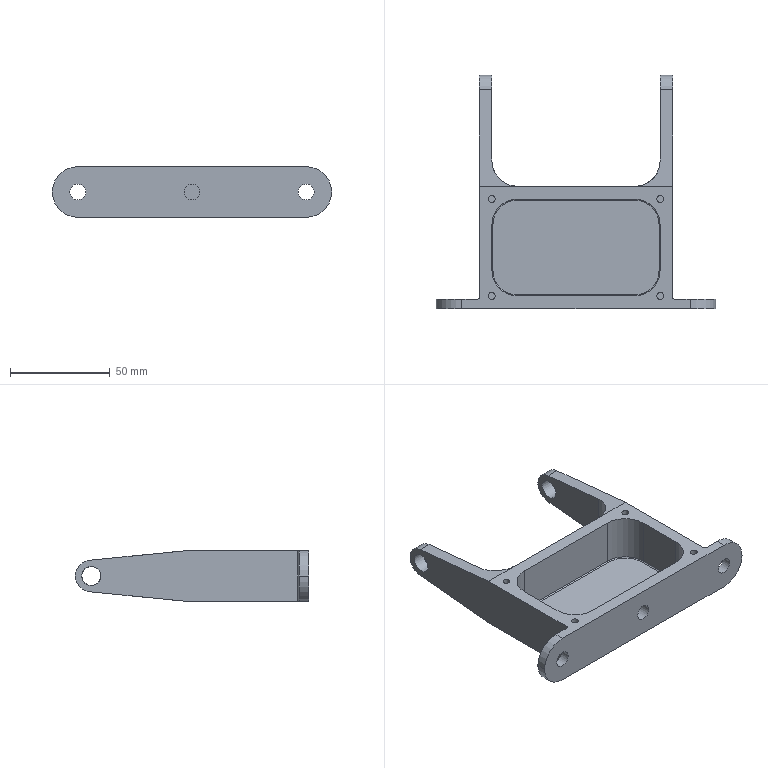Part | NX | features MG0330 trunion parts 24(steering fork) 2 | 1 solid | 54 faces | box 139.7 x 116.681 x 25.4 mm | volume 74432 mm3 | cylinder 27 | plane 23 | torus 4 | commonest cylinder face diameters 25.4 x10 1.016 x4 3.454 x4 7.938 x3 1.524 x2 9.525 x2
STEP:
#1=CARTESIAN_POINT('',(-29.369,-60.325,12.7));
#2=VERTEX_POINT('',#1);
#3=CARTESIAN_POINT('',(-29.369,-60.325,-10.617));
#4=VERTEX_POINT('',#3);
#5=CARTESIAN_POINT('',(-29.369,-60.325,-11.125));
#6=DIRECTION('',(0.,0.,-1.));
#7=VECTOR('',#6,1000.);
#8=LINE('',#5,#7);
#9=EDGE_CURVE('',#2,#4,#8,.T.);
#10=ORIENTED_EDGE('',*,*,#9,.T.);
#11=CARTESIAN_POINT('',(29.369,-60.325,-10.617));
#12=VERTEX_POINT('',#11);
#13=CARTESIAN_POINT('',(29.369,-60.325,-10.617));
#14=DIRECTION('',(1.,0.,0.));
#15=VECTOR('',#14,1000.);
#16=LINE('',#13,#15);
#17=EDGE_CURVE('',#4,#12,#16,.T.);
#18=ORIENTED_EDGE('',*,*,#17,.T.);
#19=CARTESIAN_POINT('',(29.369,-60.325,12.7));
#20=VERTEX_POINT('',#19);
#21=CARTESIAN_POINT('',(29.369,-60.325,12.7));
#22=DIRECTION('',(0.,0.,-1.));
#23=VECTOR('',#22,1000.);
#24=LINE('',#21,#23);
#25=EDGE_CURVE('',#12,#20,#24,.F.);
#26=ORIENTED_EDGE('',*,*,#25,.T.);
#27=CARTESIAN_POINT('',(42.069,-60.325,12.7));
#28=DIRECTION('',(1.,0.,0.));
#29=VECTOR('',#28,1000.);
#30=LINE('',#27,#29);
#31=EDGE_CURVE('',#2,#20,#30,.T.);
#32=ORIENTED_EDGE('',*,*,#31,.F.);
#33=EDGE_LOOP('',(#10,#18,#26,#32));
#34=FACE_BOUND('',#33,.T.);
#35=CARTESIAN_POINT('',(42.069,-60.325,12.7));
#36=DIRECTION('',(0.,1.,0.));
#37=DIRECTION('',(0.,0.,1.));
#38=AXIS2_PLACEMENT_3D('',#35,#36,#37);
#39=PLANE('',#38);
#40=ADVANCED_FACE('',(#34),#39,.F.);
#41=CARTESIAN_POINT('',(42.069,-73.025,12.7));
#42=VERTEX_POINT('',#41);
#43=CARTESIAN_POINT('',(42.069,-73.025,-10.617));
#44=VERTEX_POINT('',#43);
#45=CARTESIAN_POINT('',(42.069,-73.025,-11.125));
#46=DIRECTION('',(0.,0.,-1.));
#47=VECTOR('',#46,1000.);
#48=LINE('',#45,#47);
#49=EDGE_CURVE('',#42,#44,#48,.T.);
#50=ORIENTED_EDGE('',*,*,#49,.T.);
#51=CARTESIAN_POINT('',(42.069,-96.044,-10.617));
#52=VERTEX_POINT('',#51);
#53=CARTESIAN_POINT('',(42.069,-96.044,-10.617));
#54=DIRECTION('',(0.,-1.,0.));
#55=VECTOR('',#54,1000.);
#56=LINE('',#53,#55);
#57=EDGE_CURVE('',#44,#52,#56,.T.);
#58=ORIENTED_EDGE('',*,*,#57,.T.);
#59=CARTESIAN_POINT('',(42.069,-96.044,12.7));
#60=VERTEX_POINT('',#59);
#61=CARTESIAN_POINT('',(42.069,-96.044,12.7));
#62=DIRECTION('',(0.,0.,-1.));
#63=VECTOR('',#62,1000.);
#64=LINE('',#61,#63);
#65=EDGE_CURVE('',#52,#60,#64,.F.);
#66=ORIENTED_EDGE('',*,*,#65,.T.);
#67=CARTESIAN_POINT('',(42.069,-60.325,12.7));
#68=DIRECTION('',(0.,-1.,0.));
#69=VECTOR('',#68,1000.);
#70=LINE('',#67,#69);
#71=EDGE_CURVE('',#42,#60,#70,.T.);
#72=ORIENTED_EDGE('',*,*,#71,.F.);
#73=EDGE_LOOP('',(#50,#58,#66,#72));
#74=FACE_BOUND('',#73,.T.);
#75=CARTESIAN_POINT('',(42.069,-60.325,12.7));
#76=DIRECTION('',(1.,0.,0.));
#77=DIRECTION('',(0.,1.,0.));
#78=AXIS2_PLACEMENT_3D('',#75,#76,#77);
#79=PLANE('',#78);
#80=ADVANCED_FACE('',(#74),#79,.F.);
#81=CARTESIAN_POINT('',(0.,-108.744,-3.969));
#82=VERTEX_POINT('',#81);
#83=CARTESIAN_POINT('',(0.,-108.744,0.));
#84=DIRECTION('',(0.,-1.,0.));
#85=DIRECTION('',(0.,0.,-1.));
#86=AXIS2_PLACEMENT_3D('',#83,#84,#85);
#87=CIRCLE('',#86,3.969);
#88=EDGE_CURVE('',#82,#82,#87,.F.);
#89=ORIENTED_EDGE('',*,*,#88,.F.);
#90=EDGE_LOOP('',(#89));
#91=FACE_BOUND('',#90,.T.);
#92=CARTESIAN_POINT('',(29.369,-108.744,12.7));
#93=VERTEX_POINT('',#92);
#94=CARTESIAN_POINT('',(29.369,-108.744,-10.617));
#95=VERTEX_POINT('',#94);
#96=CARTESIAN_POINT('',(29.369,-108.744,-11.125));
#97=DIRECTION('',(0.,0.,-1.));
#98=VECTOR('',#97,1000.);
#99=LINE('',#96,#98);
#100=EDGE_CURVE('',#93,#95,#99,.T.);
#101=ORIENTED_EDGE('',*,*,#100,.T.);
#102=CARTESIAN_POINT('',(-29.369,-108.744,-10.617));
#103=VERTEX_POINT('',#102);
#104=CARTESIAN_POINT('',(-29.369,-108.744,-10.617));
#105=DIRECTION('',(-1.,0.,0.));
#106=VECTOR('',#105,1000.);
#107=LINE('',#104,#106);
#108=EDGE_CURVE('',#95,#103,#107,.T.);
#109=ORIENTED_EDGE('',*,*,#108,.T.);
#110=CARTESIAN_POINT('',(-29.369,-108.744,12.7));
#111=VERTEX_POINT('',#110);
#112=CARTESIAN_POINT('',(-29.369,-108.744,12.7));
#113=DIRECTION('',(0.,0.,-1.));
#114=VECTOR('',#113,1000.);
#115=LINE('',#112,#114);
#116=EDGE_CURVE('',#103,#111,#115,.F.);
#117=ORIENTED_EDGE('',*,*,#116,.T.);
#118=CARTESIAN_POINT('',(42.069,-108.744,12.7));
#119=DIRECTION('',(-1.,0.,0.));
#120=VECTOR('',#119,1000.);
#121=LINE('',#118,#120);
#122=EDGE_CURVE('',#93,#111,#121,.T.);
#123=ORIENTED_EDGE('',*,*,#122,.F.);
#124=EDGE_LOOP('',(#101,#109,#117,#123));
#125=FACE_BOUND('',#124,.T.);
#126=CARTESIAN_POINT('',(42.069,-108.744,12.7));
#127=DIRECTION('',(0.,-1.,0.));
#128=DIRECTION('',(0.,0.,-1.));
#129=AXIS2_PLACEMENT_3D('',#126,#127,#128);
#130=PLANE('',#129);
#131=ADVANCED_FACE('',(#91,#125),#130,.F.);
#132=CARTESIAN_POINT('',(57.15,-115.094,-3.969));
#133=VERTEX_POINT('',#132);
#134=CARTESIAN_POINT('',(57.15,-115.094,0.));
#135=DIRECTION('',(0.,-1.,0.));
#136=DIRECTION('',(0.,0.,-1.));
#137=AXIS2_PLACEMENT_3D('',#134,#135,#136);
#138=CIRCLE('',#137,3.969);
#139=EDGE_CURVE('',#133,#133,#138,.T.);
#140=ORIENTED_EDGE('',*,*,#139,.F.);
#141=EDGE_LOOP('',(#140));
#142=FACE_BOUND('',#141,.T.);
#143=CARTESIAN_POINT('',(-57.15,-115.094,-3.969));
#144=VERTEX_POINT('',#143);
#145=CARTESIAN_POINT('',(-57.15,-115.094,0.));
#146=DIRECTION('',(0.,-1.,0.));
#147=DIRECTION('',(0.,0.,-1.));
#148=AXIS2_PLACEMENT_3D('',#145,#146,#147);
#149=CIRCLE('',#148,3.969);
#150=EDGE_CURVE('',#144,#144,#149,.T.);
#151=ORIENTED_EDGE('',*,*,#150,.F.);
#152=EDGE_LOOP('',(#151));
#153=FACE_BOUND('',#152,.T.);
#154=CARTESIAN_POINT('',(0.,-115.094,-3.969));
#155=VERTEX_POINT('',#154);
#156=CARTESIAN_POINT('',(0.,-115.094,0.));
#157=DIRECTION('',(0.,-1.,0.));
#158=DIRECTION('',(0.,0.,-1.));
#159=AXIS2_PLACEMENT_3D('',#156,#157,#158);
#160=CIRCLE('',#159,3.969);
#161=EDGE_CURVE('',#155,#155,#160,.T.);
#162=ORIENTED_EDGE('',*,*,#161,.F.);
#163=EDGE_LOOP('',(#162));
#164=FACE_BOUND('',#163,.T.);
#165=CARTESIAN_POINT('',(-57.15,-115.094,12.7));
#166=VERTEX_POINT('',#165);
#167=CARTESIAN_POINT('',(-69.85,-115.094,0.));
#168=VERTEX_POINT('',#167);
#169=CARTESIAN_POINT('',(-57.15,-115.094,0.));
#170=DIRECTION('',(0.,1.,0.));
#171=DIRECTION('',(-1.,0.,0.));
#172=AXIS2_PLACEMENT_3D('',#169,#170,#171);
#173=CIRCLE('',#172,12.7);
#174=EDGE_CURVE('',#166,#168,#173,.F.);
#175=ORIENTED_EDGE('',*,*,#174,.T.);
#176=CARTESIAN_POINT('',(-57.15,-115.094,-12.7));
#177=VERTEX_POINT('',#176);
#178=CARTESIAN_POINT('',(-57.15,-115.094,0.));
#179=DIRECTION('',(0.,1.,0.));
#180=DIRECTION('',(-1.,0.,0.));
#181=AXIS2_PLACEMENT_3D('',#178,#179,#180);
#182=CIRCLE('',#181,12.7);
#183=EDGE_CURVE('',#168,#177,#182,.F.);
#184=ORIENTED_EDGE('',*,*,#183,.T.);
#185=CARTESIAN_POINT('',(57.15,-115.094,-12.7));
#186=VERTEX_POINT('',#185);
#187=CARTESIAN_POINT('',(0.,-115.094,-12.7));
#188=DIRECTION('',(1.,0.,0.));
#189=VECTOR('',#188,1000.);
#190=LINE('',#187,#189);
#191=EDGE_CURVE('',#177,#186,#190,.T.);
#192=ORIENTED_EDGE('',*,*,#191,.T.);
#193=CARTESIAN_POINT('',(69.85,-115.094,0.));
#194=VERTEX_POINT('',#193);
#195=CARTESIAN_POINT('',(57.15,-115.094,0.));
#196=DIRECTION('',(0.,1.,0.));
#197=DIRECTION('',(-1.,0.,0.));
#198=AXIS2_PLACEMENT_3D('',#195,#196,#197);
#199=CIRCLE('',#198,12.7);
#200=EDGE_CURVE('',#186,#194,#199,.F.);
#201=ORIENTED_EDGE('',*,*,#200,.T.);
#202=CARTESIAN_POINT('',(57.15,-115.094,12.7));
#203=VERTEX_POINT('',#202);
#204=CARTESIAN_POINT('',(57.15,-115.094,0.));
#205=DIRECTION('',(0.,1.,0.));
#206=DIRECTION('',(-1.,0.,0.));
#207=AXIS2_PLACEMENT_3D('',#204,#205,#206);
#208=CIRCLE('',#207,12.7);
#209=EDGE_CURVE('',#194,#203,#208,.F.);
#210=ORIENTED_EDGE('',*,*,#209,.T.);
#211=CARTESIAN_POINT('',(0.,-115.094,12.7));
#212=DIRECTION('',(1.,0.,0.));
#213=VECTOR('',#212,1000.);
#214=LINE('',#211,#213);
#215=EDGE_CURVE('',#166,#203,#214,.T.);
#216=ORIENTED_EDGE('',*,*,#215,.F.);
#217=EDGE_LOOP('',(#175,#184,#192,#201,#210,#216));
#218=FACE_BOUND('',#217,.T.);
#219=CARTESIAN_POINT('',(0.,-115.094,12.7));
#220=DIRECTION('',(0.,1.,0.));
#221=DIRECTION('',(-1.,0.,0.));
#222=AXIS2_PLACEMENT_3D('',#219,#220,#221);
#223=PLANE('',#222);
#224=ADVANCED_FACE('',(#142,#153,#164,#218),#223,.F.);
#225=CARTESIAN_POINT('',(57.15,-110.331,-3.969));
#226=VERTEX_POINT('',#225);
#227=CARTESIAN_POINT('',(57.15,-110.331,0.));
#228=DIRECTION('',(0.,-1.,0.));
#229=DIRECTION('',(0.,0.,-1.));
#230=AXIS2_PLACEMENT_3D('',#227,#228,#229);
#231=CIRCLE('',#230,3.969);
#232=EDGE_CURVE('',#226,#226,#231,.T.);
#233=ORIENTED_EDGE('',*,*,#232,.T.);
#234=EDGE_LOOP('',(#233));
#235=FACE_BOUND('',#234,.T.);
#236=CARTESIAN_POINT('',(57.15,-110.331,-12.7));
#237=VERTEX_POINT('',#236);
#238=CARTESIAN_POINT('',(49.181,-110.331,-12.7));
#239=VERTEX_POINT('',#238);
#240=CARTESIAN_POINT('',(69.85,-110.331,-12.7));
#241=DIRECTION('',(-1.,0.,0.));
#242=VECTOR('',#241,1000.);
#243=LINE('',#240,#242);
#244=EDGE_CURVE('',#237,#239,#243,.T.);
#245=ORIENTED_EDGE('',*,*,#244,.T.);
#246=CARTESIAN_POINT('',(49.181,-110.331,12.7));
#247=VERTEX_POINT('',#246);
#248=CARTESIAN_POINT('',(49.181,-110.331,12.7));
#249=DIRECTION('',(0.,0.,-1.));
#250=VECTOR('',#249,1000.);
#251=LINE('',#248,#250);
#252=EDGE_CURVE('',#239,#247,#251,.F.);
#253=ORIENTED_EDGE('',*,*,#252,.T.);
#254=CARTESIAN_POINT('',(57.15,-110.331,12.7));
#255=VERTEX_POINT('',#254);
#256=CARTESIAN_POINT('',(69.85,-110.331,12.7));
#257=DIRECTION('',(-1.,0.,0.));
#258=VECTOR('',#257,1000.);
#259=LINE('',#256,#258);
#260=EDGE_CURVE('',#255,#247,#259,.T.);
#261=ORIENTED_EDGE('',*,*,#260,.F.);
#262=CARTESIAN_POINT('',(69.85,-110.331,0.));
#263=VERTEX_POINT('',#262);
#264=CARTESIAN_POINT('',(57.15,-110.331,0.));
#265=DIRECTION('',(0.,-1.,0.));
#266=DIRECTION('',(0.,0.,-1.));
#267=AXIS2_PLACEMENT_3D('',#264,#265,#266);
#268=CIRCLE('',#267,12.7);
#269=EDGE_CURVE('',#255,#263,#268,.F.);
#270=ORIENTED_EDGE('',*,*,#269,.T.);
#271=CARTESIAN_POINT('',(57.15,-110.331,0.));
#272=DIRECTION('',(0.,-1.,0.));
#273=DIRECTION('',(0.,0.,-1.));
#274=AXIS2_PLACEMENT_3D('',#271,#272,#273);
#275=CIRCLE('',#274,12.7);
#276=EDGE_CURVE('',#263,#237,#275,.F.);
#277=ORIENTED_EDGE('',*,*,#276,.T.);
#278=EDGE_LOOP('',(#245,#253,#261,#270,#277));
#279=FACE_BOUND('',#278,.T.);
#280=CARTESIAN_POINT('',(69.85,-110.331,12.7));
#281=DIRECTION('',(0.,-1.,0.));
#282=DIRECTION('',(0.,0.,-1.));
#283=AXIS2_PLACEMENT_3D('',#280,#281,#282);
#284=PLANE('',#283);
#285=ADVANCED_FACE('',(#235,#279),#284,.F.);
#286=CARTESIAN_POINT('',(48.419,-6.35,4.763));
#287=VERTEX_POINT('',#286);
#288=CARTESIAN_POINT('',(48.419,-6.35,0.));
#289=DIRECTION('',(-1.,0.,0.));
#290=DIRECTION('',(0.,0.,1.));
#291=AXIS2_PLACEMENT_3D('',#288,#289,#290);
#292=CIRCLE('',#291,4.763);
#293=EDGE_CURVE('',#287,#287,#292,.T.);
#294=ORIENTED_EDGE('',*,*,#293,.T.);
#295=EDGE_LOOP('',(#294));
#296=FACE_BOUND('',#295,.T.);
#297=CARTESIAN_POINT('',(48.419,-109.569,12.7));
#298=VERTEX_POINT('',#297);
#299=CARTESIAN_POINT('',(48.419,-53.975,12.7));
#300=VERTEX_POINT('',#299);
#301=CARTESIAN_POINT('',(48.419,-110.331,12.7));
#302=DIRECTION('',(0.,1.,0.));
#303=VECTOR('',#302,1000.);
#304=LINE('',#301,#303);
#305=EDGE_CURVE('',#298,#300,#304,.T.);
#306=ORIENTED_EDGE('',*,*,#305,.F.);
#307=CARTESIAN_POINT('',(48.419,-109.569,-12.7));
#308=VERTEX_POINT('',#307);
#309=CARTESIAN_POINT('',(48.419,-109.569,-12.7));
#310=DIRECTION('',(0.,0.,-1.));
#311=VECTOR('',#310,1000.);
#312=LINE('',#309,#311);
#313=EDGE_CURVE('',#298,#308,#312,.T.);
#314=ORIENTED_EDGE('',*,*,#313,.T.);
#315=CARTESIAN_POINT('',(48.419,-53.975,-12.7));
#316=VERTEX_POINT('',#315);
#317=CARTESIAN_POINT('',(48.419,-110.331,-12.7));
#318=DIRECTION('',(0.,1.,0.));
#319=VECTOR('',#318,1000.);
#320=LINE('',#317,#319);
#321=EDGE_CURVE('',#308,#316,#320,.T.);
#322=ORIENTED_EDGE('',*,*,#321,.T.);
#323=CARTESIAN_POINT('',(48.419,-5.567,-7.899));
#324=VERTEX_POINT('',#323);
#325=CARTESIAN_POINT('',(48.419,-107.288,-17.988));
#326=DIRECTION('',(0.,0.9951,0.0987));
#327=VECTOR('',#326,1000.);
#328=LINE('',#325,#327);
#329=EDGE_CURVE('',#316,#324,#328,.T.);
#330=ORIENTED_EDGE('',*,*,#329,.T.);
#331=CARTESIAN_POINT('',(48.419,-5.567,7.899));
#332=VERTEX_POINT('',#331);
#333=CARTESIAN_POINT('',(48.419,-6.35,0.));
#334=DIRECTION('',(-1.,0.,0.));
#335=DIRECTION('',(0.,0.,1.));
#336=AXIS2_PLACEMENT_3D('',#333,#334,#335);
#337=CIRCLE('',#336,7.938);
#338=EDGE_CURVE('',#324,#332,#337,.F.);
#339=ORIENTED_EDGE('',*,*,#338,.T.);
#340=CARTESIAN_POINT('',(48.419,-109.782,18.235));
#341=DIRECTION('',(0.,-0.9951,0.0987));
#342=VECTOR('',#341,1000.);
#343=LINE('',#340,#342);
#344=EDGE_CURVE('',#332,#300,#343,.T.);
#345=ORIENTED_EDGE('',*,*,#344,.T.);
#346=EDGE_LOOP('',(#306,#314,#322,#330,#339,#345));
#347=FACE_BOUND('',#346,.T.);
#348=CARTESIAN_POINT('',(48.419,-110.331,12.7));
#349=DIRECTION('',(-1.,0.,0.));
#350=DIRECTION('',(0.,0.,1.));
#351=AXIS2_PLACEMENT_3D('',#348,#349,#350);
#352=PLANE('',#351);
#353=ADVANCED_FACE('',(#296,#347),#352,.F.);
#354=CARTESIAN_POINT('',(42.069,-1.587,0.));
#355=VERTEX_POINT('',#354);
#356=CARTESIAN_POINT('',(42.069,-6.35,0.));
#357=DIRECTION('',(1.,0.,0.));
#358=DIRECTION('',(0.,1.,0.));
#359=AXIS2_PLACEMENT_3D('',#356,#357,#358);
#360=CIRCLE('',#359,4.763);
#361=EDGE_CURVE('',#355,#355,#360,.T.);
#362=ORIENTED_EDGE('',*,*,#361,.T.);
#363=EDGE_LOOP('',(#362));
#364=FACE_BOUND('',#363,.T.);
#365=CARTESIAN_POINT('',(42.069,-5.567,7.899));
#366=VERTEX_POINT('',#365);
#367=CARTESIAN_POINT('',(42.069,-5.567,-7.899));
#368=VERTEX_POINT('',#367);
#369=CARTESIAN_POINT('',(42.069,-6.35,0.));
#370=DIRECTION('',(1.,0.,0.));
#371=DIRECTION('',(0.,1.,0.));
#372=AXIS2_PLACEMENT_3D('',#369,#370,#371);
#373=CIRCLE('',#372,7.938);
#374=EDGE_CURVE('',#366,#368,#373,.F.);
#375=ORIENTED_EDGE('',*,*,#374,.T.);
#376=CARTESIAN_POINT('',(42.069,-41.275,-11.44));
#377=VERTEX_POINT('',#376);
#378=CARTESIAN_POINT('',(42.069,5.113,-6.84));
#379=DIRECTION('',(0.,-0.9951,-0.0987));
#380=VECTOR('',#379,1000.);
#381=LINE('',#378,#380);
#382=EDGE_CURVE('',#368,#377,#381,.T.);
#383=ORIENTED_EDGE('',*,*,#382,.T.);
#384=CARTESIAN_POINT('',(42.069,-41.275,11.44));
#385=VERTEX_POINT('',#384);
#386=CARTESIAN_POINT('',(42.069,-41.275,12.7));
#387=DIRECTION('',(0.,0.,-1.));
#388=VECTOR('',#387,1000.);
#389=LINE('',#386,#388);
#390=EDGE_CURVE('',#377,#385,#389,.F.);
#391=ORIENTED_EDGE('',*,*,#390,.T.);
#392=CARTESIAN_POINT('',(42.069,2.618,7.087));
#393=DIRECTION('',(0.,0.9951,-0.0987));
#394=VECTOR('',#393,1000.);
#395=LINE('',#392,#394);
#396=EDGE_CURVE('',#385,#366,#395,.T.);
#397=ORIENTED_EDGE('',*,*,#396,.T.);
#398=EDGE_LOOP('',(#375,#383,#391,#397));
#399=FACE_BOUND('',#398,.T.);
#400=CARTESIAN_POINT('',(42.069,3.175,12.7));
#401=DIRECTION('',(1.,0.,0.));
#402=DIRECTION('',(0.,1.,0.));
#403=AXIS2_PLACEMENT_3D('',#400,#401,#402);
#404=PLANE('',#403);
#405=ADVANCED_FACE('',(#364,#399),#404,.F.);
#406=CARTESIAN_POINT('',(29.369,-53.975,12.7));
#407=VERTEX_POINT('',#406);
#408=CARTESIAN_POINT('',(-29.369,-53.975,12.7));
#409=VERTEX_POINT('',#408);
#410=CARTESIAN_POINT('',(42.069,-53.975,12.7));
#411=DIRECTION('',(-1.,0.,0.));
#412=VECTOR('',#411,1000.);
#413=LINE('',#410,#412);
#414=EDGE_CURVE('',#407,#409,#413,.T.);
#415=ORIENTED_EDGE('',*,*,#414,.F.);
#416=CARTESIAN_POINT('',(29.369,-53.975,-12.7));
#417=VERTEX_POINT('',#416);
#418=CARTESIAN_POINT('',(29.369,-53.975,-12.7));
#419=DIRECTION('',(0.,0.,-1.));
#420=VECTOR('',#419,1000.);
#421=LINE('',#418,#420);
#422=EDGE_CURVE('',#407,#417,#421,.T.);
#423=ORIENTED_EDGE('',*,*,#422,.T.);
#424=CARTESIAN_POINT('',(-29.369,-53.975,-12.7));
#425=VERTEX_POINT('',#424);
#426=CARTESIAN_POINT('',(42.069,-53.975,-12.7));
#427=DIRECTION('',(-1.,0.,0.));
#428=VECTOR('',#427,1000.);
#429=LINE('',#426,#428);
#430=EDGE_CURVE('',#417,#425,#429,.T.);
#431=ORIENTED_EDGE('',*,*,#430,.T.);
#432=CARTESIAN_POINT('',(-29.369,-53.975,12.7));
#433=DIRECTION('',(0.,0.,-1.));
#434=VECTOR('',#433,1000.);
#435=LINE('',#432,#434);
#436=EDGE_CURVE('',#425,#409,#435,.F.);
#437=ORIENTED_EDGE('',*,*,#436,.T.);
#438=EDGE_LOOP('',(#415,#423,#431,#437));
#439=FACE_BOUND('',#438,.T.);
#440=CARTESIAN_POINT('',(42.069,-53.975,12.7));
#441=DIRECTION('',(0.,-1.,0.));
#442=DIRECTION('',(1.,0.,0.));
#443=AXIS2_PLACEMENT_3D('',#440,#441,#442);
#444=PLANE('',#443);
#445=ADVANCED_FACE('',(#439),#444,.F.);
#446=CARTESIAN_POINT('',(-43.796,-60.325,12.7));
#447=VERTEX_POINT('',#446);
#448=CARTESIAN_POINT('',(-42.069,-60.325,12.7));
#449=DIRECTION('',(0.,0.,-1.));
#450=DIRECTION('',(-1.,0.,0.));
#451=AXIS2_PLACEMENT_3D('',#448,#449,#450);
#452=CIRCLE('',#451,1.727);
#453=EDGE_CURVE('',#447,#447,#452,.F.);
#454=ORIENTED_EDGE('',*,*,#453,.F.);
#455=EDGE_LOOP('',(#454));
#456=FACE_BOUND('',#455,.T.);
#457=CARTESIAN_POINT('',(40.342,-60.325,12.7));
#458=VERTEX_POINT('',#457);
#459=CARTESIAN_POINT('',(42.069,-60.325,12.7));
#460=DIRECTION('',(0.,0.,-1.));
#461=DIRECTION('',(-1.,0.,0.));
#462=AXIS2_PLACEMENT_3D('',#459,#460,#461);
#463=CIRCLE('',#462,1.727);
#464=EDGE_CURVE('',#458,#458,#463,.F.);
#465=ORIENTED_EDGE('',*,*,#464,.F.);
#466=EDGE_LOOP('',(#465));
#467=FACE_BOUND('',#466,.T.);
#468=CARTESIAN_POINT('',(40.342,-108.744,12.7));
#469=VERTEX_POINT('',#468);
#470=CARTESIAN_POINT('',(42.069,-108.744,12.7));
#471=DIRECTION('',(0.,0.,-1.));
#472=DIRECTION('',(-1.,0.,0.));
#473=AXIS2_PLACEMENT_3D('',#470,#471,#472);
#474=CIRCLE('',#473,1.727);
#475=EDGE_CURVE('',#469,#469,#474,.F.);
#476=ORIENTED_EDGE('',*,*,#475,.F.);
#477=EDGE_LOOP('',(#476));
#478=FACE_BOUND('',#477,.T.);
#479=CARTESIAN_POINT('',(-43.796,-108.744,12.7));
#480=VERTEX_POINT('',#479);
#481=CARTESIAN_POINT('',(-42.069,-108.744,12.7));
#482=DIRECTION('',(0.,0.,-1.));
#483=DIRECTION('',(-1.,0.,0.));
#484=AXIS2_PLACEMENT_3D('',#481,#482,#483);
#485=CIRCLE('',#484,1.727);
#486=EDGE_CURVE('',#480,#480,#485,.F.);
#487=ORIENTED_EDGE('',*,*,#486,.F.);
#488=EDGE_LOOP('',(#487));
#489=FACE_BOUND('',#488,.T.);
#490=ORIENTED_EDGE('',*,*,#260,.T.);
#491=CARTESIAN_POINT('',(49.181,-109.569,12.7));
#492=DIRECTION('',(0.,0.,-1.));
#493=DIRECTION('',(-1.,0.,0.));
#494=AXIS2_PLACEMENT_3D('',#491,#492,#493);
#495=CIRCLE('',#494,0.762);
#496=EDGE_CURVE('',#247,#298,#495,.T.);
#497=ORIENTED_EDGE('',*,*,#496,.T.);
#498=ORIENTED_EDGE('',*,*,#305,.T.);
#499=CARTESIAN_POINT('',(590.751,-53.975,12.7));
#500=DIRECTION('',(-1.,0.,0.));
#501=VECTOR('',#500,1000.);
#502=LINE('',#499,#501);
#503=EDGE_CURVE('',#300,#407,#502,.T.);
#504=ORIENTED_EDGE('',*,*,#503,.T.);
#505=ORIENTED_EDGE('',*,*,#414,.T.);
#506=CARTESIAN_POINT('',(-48.419,-53.975,12.7));
#507=VERTEX_POINT('',#506);
#508=CARTESIAN_POINT('',(590.751,-53.975,12.7));
#509=DIRECTION('',(-1.,0.,0.));
#510=VECTOR('',#509,1000.);
#511=LINE('',#508,#510);
#512=EDGE_CURVE('',#409,#507,#511,.T.);
#513=ORIENTED_EDGE('',*,*,#512,.T.);
#514=CARTESIAN_POINT('',(-48.419,-109.569,12.7));
#515=VERTEX_POINT('',#514);
#516=CARTESIAN_POINT('',(-48.419,-110.331,12.7));
#517=DIRECTION('',(0.,1.,0.));
#518=VECTOR('',#517,1000.);
#519=LINE('',#516,#518);
#520=EDGE_CURVE('',#515,#507,#519,.T.);
#521=ORIENTED_EDGE('',*,*,#520,.F.);
#522=CARTESIAN_POINT('',(-49.181,-110.331,12.7));
#523=VERTEX_POINT('',#522);
#524=CARTESIAN_POINT('',(-49.181,-109.569,12.7));
#525=DIRECTION('',(0.,0.,-1.));
#526=DIRECTION('',(-1.,0.,0.));
#527=AXIS2_PLACEMENT_3D('',#524,#525,#526);
#528=CIRCLE('',#527,0.762);
#529=EDGE_CURVE('',#515,#523,#528,.T.);
#530=ORIENTED_EDGE('',*,*,#529,.T.);
#531=CARTESIAN_POINT('',(-57.15,-110.331,12.7));
#532=VERTEX_POINT('',#531);
#533=CARTESIAN_POINT('',(-69.85,-110.331,12.7));
#534=DIRECTION('',(1.,0.,0.));
#535=VECTOR('',#534,1000.);
#536=LINE('',#533,#535);
#537=EDGE_CURVE('',#532,#523,#536,.T.);
#538=ORIENTED_EDGE('',*,*,#537,.F.);
#539=CARTESIAN_POINT('',(-57.15,-115.094,12.7));
#540=DIRECTION('',(0.,1.,0.));
#541=VECTOR('',#540,1000.);
#542=LINE('',#539,#541);
#543=EDGE_CURVE('',#532,#166,#542,.F.);
#544=ORIENTED_EDGE('',*,*,#543,.T.);
#545=ORIENTED_EDGE('',*,*,#215,.T.);
#546=CARTESIAN_POINT('',(57.15,-115.094,12.7));
#547=DIRECTION('',(0.,1.,0.));
#548=VECTOR('',#547,1000.);
#549=LINE('',#546,#548);
#550=EDGE_CURVE('',#203,#255,#549,.T.);
#551=ORIENTED_EDGE('',*,*,#550,.T.);
#552=EDGE_LOOP('',(#490,#497,#498,#504,#505,#513,#521,#530,#538,#544,#545,#551));
#553=FACE_BOUND('',#552,.T.);
#554=ORIENTED_EDGE('',*,*,#71,.T.);
#555=CARTESIAN_POINT('',(29.369,-96.044,12.7));
#556=DIRECTION('',(0.,0.,-1.));
#557=DIRECTION('',(-1.,0.,0.));
#558=AXIS2_PLACEMENT_3D('',#555,#556,#557);
#559=CIRCLE('',#558,12.7);
#560=EDGE_CURVE('',#60,#93,#559,.T.);
#561=ORIENTED_EDGE('',*,*,#560,.T.);
#562=ORIENTED_EDGE('',*,*,#122,.T.);
#563=CARTESIAN_POINT('',(-42.069,-96.044,12.7));
#564=VERTEX_POINT('',#563);
#565=CARTESIAN_POINT('',(-29.369,-96.044,12.7));
#566=DIRECTION('',(0.,0.,-1.));
#567=DIRECTION('',(-1.,0.,0.));
#568=AXIS2_PLACEMENT_3D('',#565,#566,#567);
#569=CIRCLE('',#568,12.7);
#570=EDGE_CURVE('',#111,#564,#569,.T.);
#571=ORIENTED_EDGE('',*,*,#570,.T.);
#572=CARTESIAN_POINT('',(-42.069,-73.025,12.7));
#573=VERTEX_POINT('',#572);
#574=CARTESIAN_POINT('',(-42.069,-60.325,12.7));
#575=DIRECTION('',(0.,-1.,0.));
#576=VECTOR('',#575,1000.);
#577=LINE('',#574,#576);
#578=EDGE_CURVE('',#573,#564,#577,.T.);
#579=ORIENTED_EDGE('',*,*,#578,.F.);
#580=CARTESIAN_POINT('',(-29.369,-73.025,12.7));
#581=DIRECTION('',(0.,0.,-1.));
#582=DIRECTION('',(-1.,0.,0.));
#583=AXIS2_PLACEMENT_3D('',#580,#581,#582);
#584=CIRCLE('',#583,12.7);
#585=EDGE_CURVE('',#573,#2,#584,.T.);
#586=ORIENTED_EDGE('',*,*,#585,.T.);
#587=ORIENTED_EDGE('',*,*,#31,.T.);
#588=CARTESIAN_POINT('',(29.369,-73.025,12.7));
#589=DIRECTION('',(0.,0.,-1.));
#590=DIRECTION('',(-1.,0.,0.));
#591=AXIS2_PLACEMENT_3D('',#588,#589,#590);
#592=CIRCLE('',#591,12.7);
#593=EDGE_CURVE('',#20,#42,#592,.T.);
#594=ORIENTED_EDGE('',*,*,#593,.T.);
#595=EDGE_LOOP('',(#554,#561,#562,#571,#579,#586,#587,#594));
#596=FACE_BOUND('',#595,.T.);
#597=CARTESIAN_POINT('',(0.,-115.094,12.7));
#598=DIRECTION('',(0.,0.,-1.));
#599=DIRECTION('',(-1.,0.,0.));
#600=AXIS2_PLACEMENT_3D('',#597,#598,#599);
#601=PLANE('',#600);
#602=ADVANCED_FACE('',(#456,#467,#478,#489,#553,#596),#601,.F.);
#603=CARTESIAN_POINT('',(590.751,-53.975,-12.7));
#604=DIRECTION('',(-1.,0.,0.));
#605=VECTOR('',#604,1000.);
#606=LINE('',#603,#605);
#607=EDGE_CURVE('',#316,#417,#606,.T.);
#608=ORIENTED_EDGE('',*,*,#607,.F.);
#609=ORIENTED_EDGE('',*,*,#321,.F.);
#610=CARTESIAN_POINT('',(49.181,-109.569,-12.7));
#611=DIRECTION('',(0.,0.,-1.));
#612=DIRECTION('',(-1.,0.,0.));
#613=AXIS2_PLACEMENT_3D('',#610,#611,#612);
#614=CIRCLE('',#613,0.762);
#615=EDGE_CURVE('',#308,#239,#614,.F.);
#616=ORIENTED_EDGE('',*,*,#615,.T.);
#617=ORIENTED_EDGE('',*,*,#244,.F.);
#618=CARTESIAN_POINT('',(57.15,-115.094,-12.7));
#619=DIRECTION('',(0.,1.,0.));
#620=VECTOR('',#619,1000.);
#621=LINE('',#618,#620);
#622=EDGE_CURVE('',#237,#186,#621,.F.);
#623=ORIENTED_EDGE('',*,*,#622,.T.);
#624=ORIENTED_EDGE('',*,*,#191,.F.);
#625=CARTESIAN_POINT('',(-57.15,-110.331,-12.7));
#626=VERTEX_POINT('',#625);
#627=CARTESIAN_POINT('',(-57.15,-110.331,-12.7));
#628=DIRECTION('',(0.,1.,0.));
#629=VECTOR('',#628,1000.);
#630=LINE('',#627,#629);
#631=EDGE_CURVE('',#177,#626,#630,.T.);
#632=ORIENTED_EDGE('',*,*,#631,.T.);
#633=CARTESIAN_POINT('',(-49.181,-110.331,-12.7));
#634=VERTEX_POINT('',#633);
#635=CARTESIAN_POINT('',(-69.85,-110.331,-12.7));
#636=DIRECTION('',(1.,0.,0.));
#637=VECTOR('',#636,1000.);
#638=LINE('',#635,#637);
#639=EDGE_CURVE('',#626,#634,#638,.T.);
#640=ORIENTED_EDGE('',*,*,#639,.T.);
#641=CARTESIAN_POINT('',(-48.419,-109.569,-12.7));
#642=VERTEX_POINT('',#641);
#643=CARTESIAN_POINT('',(-49.181,-109.569,-12.7));
#644=DIRECTION('',(0.,0.,-1.));
#645=DIRECTION('',(-1.,0.,0.));
#646=AXIS2_PLACEMENT_3D('',#643,#644,#645);
#647=CIRCLE('',#646,0.762);
#648=EDGE_CURVE('',#634,#642,#647,.F.);
#649=ORIENTED_EDGE('',*,*,#648,.T.);
#650=CARTESIAN_POINT('',(-48.419,-53.975,-12.7));
#651=VERTEX_POINT('',#650);
#652=CARTESIAN_POINT('',(-48.419,-110.331,-12.7));
#653=DIRECTION('',(0.,1.,0.));
#654=VECTOR('',#653,1000.);
#655=LINE('',#652,#654);
#656=EDGE_CURVE('',#642,#651,#655,.T.);
#657=ORIENTED_EDGE('',*,*,#656,.T.);
#658=CARTESIAN_POINT('',(590.751,-53.975,-12.7));
#659=DIRECTION('',(-1.,0.,0.));
#660=VECTOR('',#659,1000.);
#661=LINE('',#658,#660);
#662=EDGE_CURVE('',#425,#651,#661,.T.);
#663=ORIENTED_EDGE('',*,*,#662,.F.);
#664=ORIENTED_EDGE('',*,*,#430,.F.);
#665=EDGE_LOOP('',(#608,#609,#616,#617,#623,#624,#632,#640,#649,#657,#663,#664));
#666=FACE_BOUND('',#665,.T.);
#667=CARTESIAN_POINT('',(0.,-115.094,-12.7));
#668=DIRECTION('',(0.,0.,-1.));
#669=DIRECTION('',(-1.,0.,0.));
#670=AXIS2_PLACEMENT_3D('',#667,#668,#669);
#671=PLANE('',#670);
#672=ADVANCED_FACE('',(#666),#671,.T.);
#673=CARTESIAN_POINT('',(41.561,-96.044,-11.125));
#674=VERTEX_POINT('',#673);
#675=CARTESIAN_POINT('',(41.561,-73.025,-11.125));
#676=VERTEX_POINT('',#675);
#677=CARTESIAN_POINT('',(41.561,-73.025,-11.125));
#678=DIRECTION('',(0.,-1.,0.));
#679=VECTOR('',#678,1000.);
#680=LINE('',#677,#679);
#681=EDGE_CURVE('',#674,#676,#680,.F.);
#682=ORIENTED_EDGE('',*,*,#681,.T.);
#683=CARTESIAN_POINT('',(29.369,-60.833,-11.125));
#684=VERTEX_POINT('',#683);
#685=CARTESIAN_POINT('',(29.369,-73.025,-11.125));
#686=DIRECTION('',(0.,0.,-1.));
#687=DIRECTION('',(-1.,0.,0.));
#688=AXIS2_PLACEMENT_3D('',#685,#686,#687);
#689=CIRCLE('',#688,12.192);
#690=EDGE_CURVE('',#676,#684,#689,.F.);
#691=ORIENTED_EDGE('',*,*,#690,.T.);
#692=CARTESIAN_POINT('',(-29.369,-60.833,-11.125));
#693=VERTEX_POINT('',#692);
#694=CARTESIAN_POINT('',(-29.369,-60.833,-11.125));
#695=DIRECTION('',(1.,0.,0.));
#696=VECTOR('',#695,1000.);
#697=LINE('',#694,#696);
#698=EDGE_CURVE('',#684,#693,#697,.F.);
#699=ORIENTED_EDGE('',*,*,#698,.T.);
#700=CARTESIAN_POINT('',(-41.561,-73.025,-11.125));
#701=VERTEX_POINT('',#700);
#702=CARTESIAN_POINT('',(-29.369,-73.025,-11.125));
#703=DIRECTION('',(0.,0.,-1.));
#704=DIRECTION('',(-1.,0.,0.));
#705=AXIS2_PLACEMENT_3D('',#702,#703,#704);
#706=CIRCLE('',#705,12.192);
#707=EDGE_CURVE('',#693,#701,#706,.F.);
#708=ORIENTED_EDGE('',*,*,#707,.T.);
#709=CARTESIAN_POINT('',(-41.561,-96.044,-11.125));
#710=VERTEX_POINT('',#709);
#711=CARTESIAN_POINT('',(-41.561,-96.044,-11.125));
#712=DIRECTION('',(0.,-1.,0.));
#713=VECTOR('',#712,1000.);
#714=LINE('',#711,#713);
#715=EDGE_CURVE('',#701,#710,#714,.T.);
#716=ORIENTED_EDGE('',*,*,#715,.T.);
#717=CARTESIAN_POINT('',(-29.369,-108.236,-11.125));
#718=VERTEX_POINT('',#717);
#719=CARTESIAN_POINT('',(-29.369,-96.044,-11.125));
#720=DIRECTION('',(0.,0.,-1.));
#721=DIRECTION('',(-1.,0.,0.));
#722=AXIS2_PLACEMENT_3D('',#719,#720,#721);
#723=CIRCLE('',#722,12.192);
#724=EDGE_CURVE('',#710,#718,#723,.F.);
#725=ORIENTED_EDGE('',*,*,#724,.T.);
#726=CARTESIAN_POINT('',(29.369,-108.236,-11.125));
#727=VERTEX_POINT('',#726);
#728=CARTESIAN_POINT('',(29.369,-108.236,-11.125));
#729=DIRECTION('',(-1.,0.,0.));
#730=VECTOR('',#729,1000.);
#731=LINE('',#728,#730);
#732=EDGE_CURVE('',#718,#727,#731,.F.);
#733=ORIENTED_EDGE('',*,*,#732,.T.);
#734=CARTESIAN_POINT('',(29.369,-96.044,-11.125));
#735=DIRECTION('',(0.,0.,-1.));
#736=DIRECTION('',(-1.,0.,0.));
#737=AXIS2_PLACEMENT_3D('',#734,#735,#736);
#738=CIRCLE('',#737,12.192);
#739=EDGE_CURVE('',#727,#674,#738,.F.);
#740=ORIENTED_EDGE('',*,*,#739,.T.);
#741=EDGE_LOOP('',(#682,#691,#699,#708,#716,#725,#733,#740));
#742=FACE_BOUND('',#741,.T.);
#743=CARTESIAN_POINT('',(42.069,-108.744,-11.125));
#744=DIRECTION('',(0.,0.,-1.));
#745=DIRECTION('',(-1.,0.,0.));
#746=AXIS2_PLACEMENT_3D('',#743,#744,#745);
#747=PLANE('',#746);
#748=ADVANCED_FACE('',(#742),#747,.F.);
#749=CARTESIAN_POINT('',(-42.069,-96.044,-10.617));
#750=VERTEX_POINT('',#749);
#751=CARTESIAN_POINT('',(-42.069,-96.044,-11.125));
#752=DIRECTION('',(0.,0.,-1.));
#753=VECTOR('',#752,1000.);
#754=LINE('',#751,#753);
#755=EDGE_CURVE('',#564,#750,#754,.T.);
#756=ORIENTED_EDGE('',*,*,#755,.T.);
#757=CARTESIAN_POINT('',(-42.069,-73.025,-10.617));
#758=VERTEX_POINT('',#757);
#759=CARTESIAN_POINT('',(-42.069,-73.025,-10.617));
#760=DIRECTION('',(0.,-1.,0.));
#761=VECTOR('',#760,1000.);
#762=LINE('',#759,#761);
#763=EDGE_CURVE('',#750,#758,#762,.F.);
#764=ORIENTED_EDGE('',*,*,#763,.T.);
#765=CARTESIAN_POINT('',(-42.069,-73.025,12.7));
#766=DIRECTION('',(0.,0.,-1.));
#767=VECTOR('',#766,1000.);
#768=LINE('',#765,#767);
#769=EDGE_CURVE('',#758,#573,#768,.F.);
#770=ORIENTED_EDGE('',*,*,#769,.T.);
#771=ORIENTED_EDGE('',*,*,#578,.T.);
#772=EDGE_LOOP('',(#756,#764,#770,#771));
#773=FACE_BOUND('',#772,.T.);
#774=CARTESIAN_POINT('',(-42.069,-60.325,12.7));
#775=DIRECTION('',(-1.,0.,0.));
#776=DIRECTION('',(0.,1.,0.));
#777=AXIS2_PLACEMENT_3D('',#774,#775,#776);
#778=PLANE('',#777);
#779=ADVANCED_FACE('',(#773),#778,.F.);
#780=CARTESIAN_POINT('',(-57.15,-110.331,-3.969));
#781=VERTEX_POINT('',#780);
#782=CARTESIAN_POINT('',(-57.15,-110.331,0.));
#783=DIRECTION('',(0.,-1.,0.));
#784=DIRECTION('',(0.,0.,-1.));
#785=AXIS2_PLACEMENT_3D('',#782,#783,#784);
#786=CIRCLE('',#785,3.969);
#787=EDGE_CURVE('',#781,#781,#786,.T.);
#788=ORIENTED_EDGE('',*,*,#787,.T.);
#789=EDGE_LOOP('',(#788));
#790=FACE_BOUND('',#789,.T.);
#791=ORIENTED_EDGE('',*,*,#537,.T.);
#792=CARTESIAN_POINT('',(-49.181,-110.331,-12.7));
#793=DIRECTION('',(0.,0.,-1.));
#794=VECTOR('',#793,1000.);
#795=LINE('',#792,#794);
#796=EDGE_CURVE('',#523,#634,#795,.T.);
#797=ORIENTED_EDGE('',*,*,#796,.T.);
#798=ORIENTED_EDGE('',*,*,#639,.F.);
#799=CARTESIAN_POINT('',(-69.85,-110.331,0.));
#800=VERTEX_POINT('',#799);
#801=CARTESIAN_POINT('',(-57.15,-110.331,0.));
#802=DIRECTION('',(0.,-1.,0.));
#803=DIRECTION('',(0.,0.,-1.));
#804=AXIS2_PLACEMENT_3D('',#801,#802,#803);
#805=CIRCLE('',#804,12.7);
#806=EDGE_CURVE('',#626,#800,#805,.F.);
#807=ORIENTED_EDGE('',*,*,#806,.T.);
#808=CARTESIAN_POINT('',(-57.15,-110.331,0.));
#809=DIRECTION('',(0.,-1.,0.));
#810=DIRECTION('',(0.,0.,-1.));
#811=AXIS2_PLACEMENT_3D('',#808,#809,#810);
#812=CIRCLE('',#811,12.7);
#813=EDGE_CURVE('',#800,#532,#812,.F.);
#814=ORIENTED_EDGE('',*,*,#813,.T.);
#815=EDGE_LOOP('',(#791,#797,#798,#807,#814));
#816=FACE_BOUND('',#815,.T.);
#817=CARTESIAN_POINT('',(-69.85,-110.331,12.7));
#818=DIRECTION('',(0.,-1.,0.));
#819=DIRECTION('',(0.,0.,-1.));
#820=AXIS2_PLACEMENT_3D('',#817,#818,#819);
#821=PLANE('',#820);
#822=ADVANCED_FACE('',(#790,#816),#821,.F.);
#823=CARTESIAN_POINT('',(-48.419,-6.35,-4.763));
#824=VERTEX_POINT('',#823);
#825=CARTESIAN_POINT('',(-48.419,-6.35,0.));
#826=DIRECTION('',(1.,0.,0.));
#827=DIRECTION('',(0.,0.,-1.));
#828=AXIS2_PLACEMENT_3D('',#825,#826,#827);
#829=CIRCLE('',#828,4.763);
#830=EDGE_CURVE('',#824,#824,#829,.T.);
#831=ORIENTED_EDGE('',*,*,#830,.T.);
#832=EDGE_LOOP('',(#831));
#833=FACE_BOUND('',#832,.T.);
#834=ORIENTED_EDGE('',*,*,#656,.F.);
#835=CARTESIAN_POINT('',(-48.419,-109.569,12.7));
#836=DIRECTION('',(0.,0.,-1.));
#837=VECTOR('',#836,1000.);
#838=LINE('',#835,#837);
#839=EDGE_CURVE('',#642,#515,#838,.F.);
#840=ORIENTED_EDGE('',*,*,#839,.T.);
#841=ORIENTED_EDGE('',*,*,#520,.T.);
#842=CARTESIAN_POINT('',(-48.419,-5.567,7.899));
#843=VERTEX_POINT('',#842);
#844=CARTESIAN_POINT('',(-48.419,-109.782,18.235));
#845=DIRECTION('',(0.,0.9951,-0.0987));
#846=VECTOR('',#845,1000.);
#847=LINE('',#844,#846);
#848=EDGE_CURVE('',#507,#843,#847,.T.);
#849=ORIENTED_EDGE('',*,*,#848,.T.);
#850=CARTESIAN_POINT('',(-48.419,-5.567,-7.899));
#851=VERTEX_POINT('',#850);
#852=CARTESIAN_POINT('',(-48.419,-6.35,0.));
#853=DIRECTION('',(1.,0.,0.));
#854=DIRECTION('',(0.,0.,-1.));
#855=AXIS2_PLACEMENT_3D('',#852,#853,#854);
#856=CIRCLE('',#855,7.938);
#857=EDGE_CURVE('',#843,#851,#856,.F.);
#858=ORIENTED_EDGE('',*,*,#857,.T.);
#859=CARTESIAN_POINT('',(-48.419,-107.288,-17.988));
#860=DIRECTION('',(0.,-0.9951,-0.0987));
#861=VECTOR('',#860,1000.);
#862=LINE('',#859,#861);
#863=EDGE_CURVE('',#851,#651,#862,.T.);
#864=ORIENTED_EDGE('',*,*,#863,.T.);
#865=EDGE_LOOP('',(#834,#840,#841,#849,#858,#864));
#866=FACE_BOUND('',#865,.T.);
#867=CARTESIAN_POINT('',(-48.419,-110.331,12.7));
#868=DIRECTION('',(1.,0.,0.));
#869=DIRECTION('',(0.,0.,1.));
#870=AXIS2_PLACEMENT_3D('',#867,#868,#869);
#871=PLANE('',#870);
#872=ADVANCED_FACE('',(#833,#866),#871,.F.);
#873=CARTESIAN_POINT('',(-42.069,-11.113,0.));
#874=VERTEX_POINT('',#873);
#875=CARTESIAN_POINT('',(-42.069,-6.35,0.));
#876=DIRECTION('',(-1.,0.,0.));
#877=DIRECTION('',(0.,-1.,0.));
#878=AXIS2_PLACEMENT_3D('',#875,#876,#877);
#879=CIRCLE('',#878,4.763);
#880=EDGE_CURVE('',#874,#874,#879,.T.);
#881=ORIENTED_EDGE('',*,*,#880,.T.);
#882=EDGE_LOOP('',(#881));
#883=FACE_BOUND('',#882,.T.);
#884=CARTESIAN_POINT('',(-42.069,-41.275,11.44));
#885=VERTEX_POINT('',#884);
#886=CARTESIAN_POINT('',(-42.069,-41.275,-11.44));
#887=VERTEX_POINT('',#886);
#888=CARTESIAN_POINT('',(-42.069,-41.275,-12.7));
#889=DIRECTION('',(0.,0.,-1.));
#890=VECTOR('',#889,1000.);
#891=LINE('',#888,#890);
#892=EDGE_CURVE('',#885,#887,#891,.T.);
#893=ORIENTED_EDGE('',*,*,#892,.T.);
#894=CARTESIAN_POINT('',(-42.069,-5.567,-7.899));
#895=VERTEX_POINT('',#894);
#896=CARTESIAN_POINT('',(-42.069,5.113,-6.84));
#897=DIRECTION('',(0.,0.9951,0.0987));
#898=VECTOR('',#897,1000.);
#899=LINE('',#896,#898);
#900=EDGE_CURVE('',#887,#895,#899,.T.);
#901=ORIENTED_EDGE('',*,*,#900,.T.);
#902=CARTESIAN_POINT('',(-42.069,-5.567,7.899));
#903=VERTEX_POINT('',#902);
#904=CARTESIAN_POINT('',(-42.069,-6.35,0.));
#905=DIRECTION('',(-1.,0.,0.));
#906=DIRECTION('',(0.,-1.,0.));
#907=AXIS2_PLACEMENT_3D('',#904,#905,#906);
#908=CIRCLE('',#907,7.938);
#909=EDGE_CURVE('',#895,#903,#908,.F.);
#910=ORIENTED_EDGE('',*,*,#909,.T.);
#911=CARTESIAN_POINT('',(-42.069,2.618,7.087));
#912=DIRECTION('',(0.,-0.9951,0.0987));
#913=VECTOR('',#912,1000.);
#914=LINE('',#911,#913);
#915=EDGE_CURVE('',#903,#885,#914,.T.);
#916=ORIENTED_EDGE('',*,*,#915,.T.);
#917=EDGE_LOOP('',(#893,#901,#910,#916));
#918=FACE_BOUND('',#917,.T.);
#919=CARTESIAN_POINT('',(-42.069,3.175,12.7));
#920=DIRECTION('',(-1.,0.,0.));
#921=DIRECTION('',(0.,1.,0.));
#922=AXIS2_PLACEMENT_3D('',#919,#920,#921);
#923=PLANE('',#922);
#924=ADVANCED_FACE('',(#883,#918),#923,.F.);
#925=ORIENTED_EDGE('',*,*,#88,.T.);
#926=EDGE_LOOP('',(#925));
#927=FACE_BOUND('',#926,.T.);
#928=ORIENTED_EDGE('',*,*,#161,.T.);
#929=EDGE_LOOP('',(#928));
#930=FACE_BOUND('',#929,.T.);
#931=CARTESIAN_POINT('',(0.,-97.518,0.));
#932=DIRECTION('',(0.,-1.,0.));
#933=DIRECTION('',(0.,0.,-1.));
#934=AXIS2_PLACEMENT_3D('',#931,#932,#933);
#935=CYLINDRICAL_SURFACE('',#934,3.969);
#936=ADVANCED_FACE('',(#927,#930),#935,.F.);
#937=ORIENTED_EDGE('',*,*,#150,.T.);
#938=EDGE_LOOP('',(#937));
#939=FACE_BOUND('',#938,.T.);
#940=ORIENTED_EDGE('',*,*,#787,.F.);
#941=EDGE_LOOP('',(#940));
#942=FACE_BOUND('',#941,.T.);
#943=CARTESIAN_POINT('',(-57.15,-97.518,0.));
#944=DIRECTION('',(0.,-1.,0.));
#945=DIRECTION('',(0.,0.,-1.));
#946=AXIS2_PLACEMENT_3D('',#943,#944,#945);
#947=CYLINDRICAL_SURFACE('',#946,3.969);
#948=ADVANCED_FACE('',(#939,#942),#947,.F.);
#949=ORIENTED_EDGE('',*,*,#139,.T.);
#950=EDGE_LOOP('',(#949));
#951=FACE_BOUND('',#950,.T.);
#952=ORIENTED_EDGE('',*,*,#232,.F.);
#953=EDGE_LOOP('',(#952));
#954=FACE_BOUND('',#953,.T.);
#955=CARTESIAN_POINT('',(57.15,-97.518,0.));
#956=DIRECTION('',(0.,-1.,0.));
#957=DIRECTION('',(0.,0.,-1.));
#958=AXIS2_PLACEMENT_3D('',#955,#956,#957);
#959=CYLINDRICAL_SURFACE('',#958,3.969);
#960=ADVANCED_FACE('',(#951,#954),#959,.F.);
#961=CARTESIAN_POINT('',(-69.85,-115.094,0.));
#962=DIRECTION('',(0.,1.,0.));
#963=VECTOR('',#962,1000.);
#964=LINE('',#961,#963);
#965=EDGE_CURVE('',#168,#800,#964,.T.);
#966=ORIENTED_EDGE('',*,*,#965,.F.);
#967=ORIENTED_EDGE('',*,*,#174,.F.);
#968=ORIENTED_EDGE('',*,*,#543,.F.);
#969=ORIENTED_EDGE('',*,*,#813,.F.);
#970=EDGE_LOOP('',(#966,#967,#968,#969));
#971=FACE_BOUND('',#970,.T.);
#972=CARTESIAN_POINT('',(-57.15,-115.094,0.));
#973=DIRECTION('',(0.,1.,0.));
#974=DIRECTION('',(0.,0.,1.));
#975=AXIS2_PLACEMENT_3D('',#972,#973,#974);
#976=CYLINDRICAL_SURFACE('',#975,12.7);
#977=ADVANCED_FACE('',(#971),#976,.T.);
#978=ORIENTED_EDGE('',*,*,#183,.F.);
#979=ORIENTED_EDGE('',*,*,#965,.T.);
#980=ORIENTED_EDGE('',*,*,#806,.F.);
#981=ORIENTED_EDGE('',*,*,#631,.F.);
#982=EDGE_LOOP('',(#978,#979,#980,#981));
#983=FACE_BOUND('',#982,.T.);
#984=CARTESIAN_POINT('',(-57.15,-115.094,0.));
#985=DIRECTION('',(0.,-1.,0.));
#986=DIRECTION('',(0.,0.,-1.));
#987=AXIS2_PLACEMENT_3D('',#984,#985,#986);
#988=CYLINDRICAL_SURFACE('',#987,12.7);
#989=ADVANCED_FACE('',(#983),#988,.T.);
#990=ORIENTED_EDGE('',*,*,#550,.F.);
#991=ORIENTED_EDGE('',*,*,#209,.F.);
#992=CARTESIAN_POINT('',(69.85,-115.094,0.));
#993=DIRECTION('',(0.,1.,0.));
#994=VECTOR('',#993,1000.);
#995=LINE('',#992,#994);
#996=EDGE_CURVE('',#263,#194,#995,.F.);
#997=ORIENTED_EDGE('',*,*,#996,.F.);
#998=ORIENTED_EDGE('',*,*,#269,.F.);
#999=EDGE_LOOP('',(#990,#991,#997,#998));
#1000=FACE_BOUND('',#999,.T.);
#1001=CARTESIAN_POINT('',(57.15,-115.094,0.));
#1002=DIRECTION('',(0.,1.,0.));
#1003=DIRECTION('',(0.,0.,1.));
#1004=AXIS2_PLACEMENT_3D('',#1001,#1002,#1003);
#1005=CYLINDRICAL_SURFACE('',#1004,12.7);
#1006=ADVANCED_FACE('',(#1000),#1005,.T.);
#1007=ORIENTED_EDGE('',*,*,#200,.F.);
#1008=ORIENTED_EDGE('',*,*,#622,.F.);
#1009=ORIENTED_EDGE('',*,*,#276,.F.);
#1010=ORIENTED_EDGE('',*,*,#996,.T.);
#1011=EDGE_LOOP('',(#1007,#1008,#1009,#1010));
#1012=FACE_BOUND('',#1011,.T.);
#1013=CARTESIAN_POINT('',(57.15,-115.094,0.));
#1014=DIRECTION('',(0.,-1.,0.));
#1015=DIRECTION('',(0.,0.,-1.));
#1016=AXIS2_PLACEMENT_3D('',#1013,#1014,#1015);
#1017=CYLINDRICAL_SURFACE('',#1016,12.7);
#1018=ADVANCED_FACE('',(#1012),#1017,.T.);
#1019=ORIENTED_EDGE('',*,*,#390,.F.);
#1020=CARTESIAN_POINT('',(29.369,-41.275,-11.44));
#1021=DIRECTION('',(0.,-0.0987,0.9951));
#1022=DIRECTION('',(0.,0.9951,0.0987));
#1023=AXIS2_PLACEMENT_3D('',#1020,#1021,#1022);
#1024=ELLIPSE('',#1023,12.762,12.7);
#1025=EDGE_CURVE('',#377,#417,#1024,.F.);
#1026=ORIENTED_EDGE('',*,*,#1025,.T.);
#1027=ORIENTED_EDGE('',*,*,#422,.F.);
#1028=CARTESIAN_POINT('',(29.369,-41.275,11.44));
#1029=DIRECTION('',(0.,-0.0987,-0.9951));
#1030=DIRECTION('',(0.,-0.9951,0.0987));
#1031=AXIS2_PLACEMENT_3D('',#1028,#1029,#1030);
#1032=ELLIPSE('',#1031,12.762,12.7);
#1033=EDGE_CURVE('',#407,#385,#1032,.F.);
#1034=ORIENTED_EDGE('',*,*,#1033,.T.);
#1035=EDGE_LOOP('',(#1019,#1026,#1027,#1034));
#1036=FACE_BOUND('',#1035,.T.);
#1037=CARTESIAN_POINT('',(29.369,-41.275,12.7));
#1038=DIRECTION('',(0.,0.,1.));
#1039=DIRECTION('',(1.,0.,0.));
#1040=AXIS2_PLACEMENT_3D('',#1037,#1038,#1039);
#1041=CYLINDRICAL_SURFACE('',#1040,12.7);
#1042=ADVANCED_FACE('',(#1036),#1041,.F.);
#1043=ORIENTED_EDGE('',*,*,#436,.F.);
#1044=CARTESIAN_POINT('',(-29.369,-41.275,-11.44));
#1045=DIRECTION('',(0.,-0.0987,0.9951));
#1046=DIRECTION('',(0.,0.9951,0.0987));
#1047=AXIS2_PLACEMENT_3D('',#1044,#1045,#1046);
#1048=ELLIPSE('',#1047,12.762,12.7);
#1049=EDGE_CURVE('',#425,#887,#1048,.F.);
#1050=ORIENTED_EDGE('',*,*,#1049,.T.);
#1051=ORIENTED_EDGE('',*,*,#892,.F.);
#1052=CARTESIAN_POINT('',(-29.369,-41.275,11.44));
#1053=DIRECTION('',(0.,-0.0987,-0.9951));
#1054=DIRECTION('',(0.,-0.9951,0.0987));
#1055=AXIS2_PLACEMENT_3D('',#1052,#1053,#1054);
#1056=ELLIPSE('',#1055,12.762,12.7);
#1057=EDGE_CURVE('',#885,#409,#1056,.F.);
#1058=ORIENTED_EDGE('',*,*,#1057,.T.);
#1059=EDGE_LOOP('',(#1043,#1050,#1051,#1058));
#1060=FACE_BOUND('',#1059,.T.);
#1061=CARTESIAN_POINT('',(-29.369,-41.275,12.7));
#1062=DIRECTION('',(0.,0.,1.));
#1063=DIRECTION('',(1.,0.,0.));
#1064=AXIS2_PLACEMENT_3D('',#1061,#1062,#1063);
#1065=CYLINDRICAL_SURFACE('',#1064,12.7);
#1066=ADVANCED_FACE('',(#1060),#1065,.F.);
#1067=ORIENTED_EDGE('',*,*,#769,.F.);
#1068=CARTESIAN_POINT('',(-29.369,-73.025,-10.617));
#1069=DIRECTION('',(0.,0.,-1.));
#1070=DIRECTION('',(-1.,0.,0.));
#1071=AXIS2_PLACEMENT_3D('',#1068,#1069,#1070);
#1072=CIRCLE('',#1071,12.7);
#1073=EDGE_CURVE('',#758,#4,#1072,.T.);
#1074=ORIENTED_EDGE('',*,*,#1073,.T.);
#1075=ORIENTED_EDGE('',*,*,#9,.F.);
#1076=ORIENTED_EDGE('',*,*,#585,.F.);
#1077=EDGE_LOOP('',(#1067,#1074,#1075,#1076));
#1078=FACE_BOUND('',#1077,.T.);
#1079=CARTESIAN_POINT('',(-29.369,-73.025,12.7));
#1080=DIRECTION('',(0.,0.,1.));
#1081=DIRECTION('',(1.,0.,0.));
#1082=AXIS2_PLACEMENT_3D('',#1079,#1080,#1081);
#1083=CYLINDRICAL_SURFACE('',#1082,12.7);
#1084=ADVANCED_FACE('',(#1078),#1083,.F.);
#1085=ORIENTED_EDGE('',*,*,#25,.F.);
#1086=CARTESIAN_POINT('',(29.369,-73.025,-10.617));
#1087=DIRECTION('',(0.,0.,-1.));
#1088=DIRECTION('',(-1.,0.,0.));
#1089=AXIS2_PLACEMENT_3D('',#1086,#1087,#1088);
#1090=CIRCLE('',#1089,12.7);
#1091=EDGE_CURVE('',#12,#44,#1090,.T.);
#1092=ORIENTED_EDGE('',*,*,#1091,.T.);
#1093=ORIENTED_EDGE('',*,*,#49,.F.);
#1094=ORIENTED_EDGE('',*,*,#593,.F.);
#1095=EDGE_LOOP('',(#1085,#1092,#1093,#1094));
#1096=FACE_BOUND('',#1095,.T.);
#1097=CARTESIAN_POINT('',(29.369,-73.025,12.7));
#1098=DIRECTION('',(0.,0.,1.));
#1099=DIRECTION('',(1.,0.,0.));
#1100=AXIS2_PLACEMENT_3D('',#1097,#1098,#1099);
#1101=CYLINDRICAL_SURFACE('',#1100,12.7);
#1102=ADVANCED_FACE('',(#1096),#1101,.F.);
#1103=ORIENTED_EDGE('',*,*,#65,.F.);
#1104=CARTESIAN_POINT('',(29.369,-96.044,-10.617));
#1105=DIRECTION('',(0.,0.,-1.));
#1106=DIRECTION('',(-1.,0.,0.));
#1107=AXIS2_PLACEMENT_3D('',#1104,#1105,#1106);
#1108=CIRCLE('',#1107,12.7);
#1109=EDGE_CURVE('',#52,#95,#1108,.T.);
#1110=ORIENTED_EDGE('',*,*,#1109,.T.);
#1111=ORIENTED_EDGE('',*,*,#100,.F.);
#1112=ORIENTED_EDGE('',*,*,#560,.F.);
#1113=EDGE_LOOP('',(#1103,#1110,#1111,#1112));
#1114=FACE_BOUND('',#1113,.T.);
#1115=CARTESIAN_POINT('',(29.369,-96.044,12.7));
#1116=DIRECTION('',(0.,0.,1.));
#1117=DIRECTION('',(1.,0.,0.));
#1118=AXIS2_PLACEMENT_3D('',#1115,#1116,#1117);
#1119=CYLINDRICAL_SURFACE('',#1118,12.7);
#1120=ADVANCED_FACE('',(#1114),#1119,.F.);
#1121=ORIENTED_EDGE('',*,*,#116,.F.);
#1122=CARTESIAN_POINT('',(-29.369,-96.044,-10.617));
#1123=DIRECTION('',(0.,0.,-1.));
#1124=DIRECTION('',(-1.,0.,0.));
#1125=AXIS2_PLACEMENT_3D('',#1122,#1123,#1124);
#1126=CIRCLE('',#1125,12.7);
#1127=EDGE_CURVE('',#103,#750,#1126,.T.);
#1128=ORIENTED_EDGE('',*,*,#1127,.T.);
#1129=ORIENTED_EDGE('',*,*,#755,.F.);
#1130=ORIENTED_EDGE('',*,*,#570,.F.);
#1131=EDGE_LOOP('',(#1121,#1128,#1129,#1130));
#1132=FACE_BOUND('',#1131,.T.);
#1133=CARTESIAN_POINT('',(-29.369,-96.044,12.7));
#1134=DIRECTION('',(0.,0.,1.));
#1135=DIRECTION('',(1.,0.,0.));
#1136=AXIS2_PLACEMENT_3D('',#1133,#1134,#1135);
#1137=CYLINDRICAL_SURFACE('',#1136,12.7);
#1138=ADVANCED_FACE('',(#1132),#1137,.F.);
#1139=ORIENTED_EDGE('',*,*,#880,.F.);
#1140=EDGE_LOOP('',(#1139));
#1141=FACE_BOUND('',#1140,.T.);
#1142=ORIENTED_EDGE('',*,*,#830,.F.);
#1143=EDGE_LOOP('',(#1142));
#1144=FACE_BOUND('',#1143,.T.);
#1145=CARTESIAN_POINT('',(-80.963,-6.35,0.));
#1146=DIRECTION('',(1.,0.,0.));
#1147=DIRECTION('',(0.,0.,-1.));
#1148=AXIS2_PLACEMENT_3D('',#1145,#1146,#1147);
#1149=CYLINDRICAL_SURFACE('',#1148,4.763);
#1150=ADVANCED_FACE('',(#1141,#1144),#1149,.F.);
#1151=ORIENTED_EDGE('',*,*,#361,.F.);
#1152=EDGE_LOOP('',(#1151));
#1153=FACE_BOUND('',#1152,.T.);
#1154=ORIENTED_EDGE('',*,*,#293,.F.);
#1155=EDGE_LOOP('',(#1154));
#1156=FACE_BOUND('',#1155,.T.);
#1157=CARTESIAN_POINT('',(-80.963,-6.35,0.));
#1158=DIRECTION('',(1.,0.,0.));
#1159=DIRECTION('',(0.,0.,-1.));
#1160=AXIS2_PLACEMENT_3D('',#1157,#1158,#1159);
#1161=CYLINDRICAL_SURFACE('',#1160,4.763);
#1162=ADVANCED_FACE('',(#1153,#1156),#1161,.F.);
#1163=ORIENTED_EDGE('',*,*,#863,.F.);
#1164=CARTESIAN_POINT('',(590.751,-5.567,-7.899));
#1165=DIRECTION('',(-1.,0.,0.));
#1166=VECTOR('',#1165,1000.);
#1167=LINE('',#1164,#1166);
#1168=EDGE_CURVE('',#895,#851,#1167,.T.);
#1169=ORIENTED_EDGE('',*,*,#1168,.F.);
#1170=ORIENTED_EDGE('',*,*,#900,.F.);
#1171=ORIENTED_EDGE('',*,*,#1049,.F.);
#1172=ORIENTED_EDGE('',*,*,#662,.T.);
#1173=EDGE_LOOP('',(#1163,#1169,#1170,#1171,#1172));
#1174=FACE_BOUND('',#1173,.T.);
#1175=CARTESIAN_POINT('',(590.751,-5.567,-7.899));
#1176=DIRECTION('',(0.,-0.0987,0.9951));
#1177=DIRECTION('',(0.,-0.9951,-0.0987));
#1178=AXIS2_PLACEMENT_3D('',#1175,#1176,#1177);
#1179=PLANE('',#1178);
#1180=ADVANCED_FACE('',(#1174),#1179,.F.);
#1181=ORIENTED_EDGE('',*,*,#848,.F.);
#1182=ORIENTED_EDGE('',*,*,#512,.F.);
#1183=ORIENTED_EDGE('',*,*,#1057,.F.);
#1184=ORIENTED_EDGE('',*,*,#915,.F.);
#1185=CARTESIAN_POINT('',(590.751,-5.567,7.899));
#1186=DIRECTION('',(-1.,0.,0.));
#1187=VECTOR('',#1186,1000.);
#1188=LINE('',#1185,#1187);
#1189=EDGE_CURVE('',#903,#843,#1188,.T.);
#1190=ORIENTED_EDGE('',*,*,#1189,.T.);
#1191=EDGE_LOOP('',(#1181,#1182,#1183,#1184,#1190));
#1192=FACE_BOUND('',#1191,.T.);
#1193=CARTESIAN_POINT('',(590.751,-5.567,7.899));
#1194=DIRECTION('',(0.,-0.0987,-0.9951));
#1195=DIRECTION('',(0.,0.9951,-0.0987));
#1196=AXIS2_PLACEMENT_3D('',#1193,#1194,#1195);
#1197=PLANE('',#1196);
#1198=ADVANCED_FACE('',(#1192),#1197,.F.);
#1199=ORIENTED_EDGE('',*,*,#857,.F.);
#1200=ORIENTED_EDGE('',*,*,#1189,.F.);
#1201=ORIENTED_EDGE('',*,*,#909,.F.);
#1202=ORIENTED_EDGE('',*,*,#1168,.T.);
#1203=EDGE_LOOP('',(#1199,#1200,#1201,#1202));
#1204=FACE_BOUND('',#1203,.T.);
#1205=CARTESIAN_POINT('',(590.751,-6.35,0.));
#1206=DIRECTION('',(-1.,0.,0.));
#1207=DIRECTION('',(0.,0.,1.));
#1208=AXIS2_PLACEMENT_3D('',#1205,#1206,#1207);
#1209=CYLINDRICAL_SURFACE('',#1208,7.938);
#1210=ADVANCED_FACE('',(#1204),#1209,.T.);
#1211=ORIENTED_EDGE('',*,*,#338,.F.);
#1212=CARTESIAN_POINT('',(590.751,-5.567,-7.899));
#1213=DIRECTION('',(-1.,0.,0.));
#1214=VECTOR('',#1213,1000.);
#1215=LINE('',#1212,#1214);
#1216=EDGE_CURVE('',#324,#368,#1215,.T.);
#1217=ORIENTED_EDGE('',*,*,#1216,.T.);
#1218=ORIENTED_EDGE('',*,*,#374,.F.);
#1219=CARTESIAN_POINT('',(590.751,-5.567,7.899));
#1220=DIRECTION('',(-1.,0.,0.));
#1221=VECTOR('',#1220,1000.);
#1222=LINE('',#1219,#1221);
#1223=EDGE_CURVE('',#332,#366,#1222,.T.);
#1224=ORIENTED_EDGE('',*,*,#1223,.F.);
#1225=EDGE_LOOP('',(#1211,#1217,#1218,#1224));
#1226=FACE_BOUND('',#1225,.T.);
#1227=CARTESIAN_POINT('',(590.751,-6.35,0.));
#1228=DIRECTION('',(-1.,0.,0.));
#1229=DIRECTION('',(0.,0.,1.));
#1230=AXIS2_PLACEMENT_3D('',#1227,#1228,#1229);
#1231=CYLINDRICAL_SURFACE('',#1230,7.938);
#1232=ADVANCED_FACE('',(#1226),#1231,.T.);
#1233=ORIENTED_EDGE('',*,*,#329,.F.);
#1234=ORIENTED_EDGE('',*,*,#607,.T.);
#1235=ORIENTED_EDGE('',*,*,#1025,.F.);
#1236=ORIENTED_EDGE('',*,*,#382,.F.);
#1237=ORIENTED_EDGE('',*,*,#1216,.F.);
#1238=EDGE_LOOP('',(#1233,#1234,#1235,#1236,#1237));
#1239=FACE_BOUND('',#1238,.T.);
#1240=CARTESIAN_POINT('',(590.751,-5.567,-7.899));
#1241=DIRECTION('',(0.,-0.0987,0.9951));
#1242=DIRECTION('',(0.,-0.9951,-0.0987));
#1243=AXIS2_PLACEMENT_3D('',#1240,#1241,#1242);
#1244=PLANE('',#1243);
#1245=ADVANCED_FACE('',(#1239),#1244,.F.);
#1246=ORIENTED_EDGE('',*,*,#344,.F.);
#1247=ORIENTED_EDGE('',*,*,#1223,.T.);
#1248=ORIENTED_EDGE('',*,*,#396,.F.);
#1249=ORIENTED_EDGE('',*,*,#1033,.F.);
#1250=ORIENTED_EDGE('',*,*,#503,.F.);
#1251=EDGE_LOOP('',(#1246,#1247,#1248,#1249,#1250));
#1252=FACE_BOUND('',#1251,.T.);
#1253=CARTESIAN_POINT('',(590.751,-5.567,7.899));
#1254=DIRECTION('',(0.,-0.0987,-0.9951));
#1255=DIRECTION('',(0.,0.9951,-0.0987));
#1256=AXIS2_PLACEMENT_3D('',#1253,#1254,#1255);
#1257=PLANE('',#1256);
#1258=ADVANCED_FACE('',(#1252),#1257,.F.);
#1259=ORIENTED_EDGE('',*,*,#529,.F.);
#1260=ORIENTED_EDGE('',*,*,#839,.F.);
#1261=ORIENTED_EDGE('',*,*,#648,.F.);
#1262=ORIENTED_EDGE('',*,*,#796,.F.);
#1263=EDGE_LOOP('',(#1259,#1260,#1261,#1262));
#1264=FACE_BOUND('',#1263,.T.);
#1265=CARTESIAN_POINT('',(-49.181,-109.569,12.7));
#1266=DIRECTION('',(0.,0.,1.));
#1267=DIRECTION('',(1.,0.,0.));
#1268=AXIS2_PLACEMENT_3D('',#1265,#1266,#1267);
#1269=CYLINDRICAL_SURFACE('',#1268,0.762);
#1270=ADVANCED_FACE('',(#1264),#1269,.F.);
#1271=ORIENTED_EDGE('',*,*,#496,.F.);
#1272=ORIENTED_EDGE('',*,*,#252,.F.);
#1273=ORIENTED_EDGE('',*,*,#615,.F.);
#1274=ORIENTED_EDGE('',*,*,#313,.F.);
#1275=EDGE_LOOP('',(#1271,#1272,#1273,#1274));
#1276=FACE_BOUND('',#1275,.T.);
#1277=CARTESIAN_POINT('',(49.181,-109.569,12.7));
#1278=DIRECTION('',(0.,0.,1.));
#1279=DIRECTION('',(1.,0.,0.));
#1280=AXIS2_PLACEMENT_3D('',#1277,#1278,#1279);
#1281=CYLINDRICAL_SURFACE('',#1280,0.762);
#1282=ADVANCED_FACE('',(#1276),#1281,.F.);
#1283=CARTESIAN_POINT('',(-41.561,-96.044,-10.617));
#1284=DIRECTION('',(0.,-1.,0.));
#1285=DIRECTION('',(0.,0.,-1.));
#1286=AXIS2_PLACEMENT_3D('',#1283,#1284,#1285);
#1287=CIRCLE('',#1286,0.508);
#1288=EDGE_CURVE('',#750,#710,#1287,.T.);
#1289=ORIENTED_EDGE('',*,*,#1288,.F.);
#1290=ORIENTED_EDGE('',*,*,#1127,.F.);
#1291=CARTESIAN_POINT('',(-29.369,-108.236,-10.617));
#1292=DIRECTION('',(-1.,0.,0.));
#1293=DIRECTION('',(0.,0.,1.));
#1294=AXIS2_PLACEMENT_3D('',#1291,#1292,#1293);
#1295=CIRCLE('',#1294,0.508);
#1296=EDGE_CURVE('',#718,#103,#1295,.T.);
#1297=ORIENTED_EDGE('',*,*,#1296,.F.);
#1298=ORIENTED_EDGE('',*,*,#724,.F.);
#1299=EDGE_LOOP('',(#1289,#1290,#1297,#1298));
#1300=FACE_BOUND('',#1299,.T.);
#1301=CARTESIAN_POINT('',(-29.369,-96.044,-10.617));
#1302=DIRECTION('',(0.,0.,-1.));
#1303=DIRECTION('',(-1.,0.,0.));
#1304=AXIS2_PLACEMENT_3D('',#1301,#1302,#1303);
#1305=TOROIDAL_SURFACE('',#1304,12.192,0.508);
#1306=ADVANCED_FACE('',(#1300),#1305,.F.);
#1307=ORIENTED_EDGE('',*,*,#1296,.T.);
#1308=ORIENTED_EDGE('',*,*,#108,.F.);
#1309=CARTESIAN_POINT('',(29.369,-108.236,-10.617));
#1310=DIRECTION('',(-1.,0.,0.));
#1311=DIRECTION('',(0.,0.,1.));
#1312=AXIS2_PLACEMENT_3D('',#1309,#1310,#1311);
#1313=CIRCLE('',#1312,0.508);
#1314=EDGE_CURVE('',#727,#95,#1313,.T.);
#1315=ORIENTED_EDGE('',*,*,#1314,.F.);
#1316=ORIENTED_EDGE('',*,*,#732,.F.);
#1317=EDGE_LOOP('',(#1307,#1308,#1315,#1316));
#1318=FACE_BOUND('',#1317,.T.);
#1319=CARTESIAN_POINT('',(42.069,-108.236,-10.617));
#1320=DIRECTION('',(1.,0.,0.));
#1321=DIRECTION('',(0.,0.,-1.));
#1322=AXIS2_PLACEMENT_3D('',#1319,#1320,#1321);
#1323=CYLINDRICAL_SURFACE('',#1322,0.508);
#1324=ADVANCED_FACE('',(#1318),#1323,.F.);
#1325=ORIENTED_EDGE('',*,*,#1288,.T.);
#1326=ORIENTED_EDGE('',*,*,#715,.F.);
#1327=CARTESIAN_POINT('',(-41.561,-73.025,-10.617));
#1328=DIRECTION('',(0.,-1.,0.));
#1329=DIRECTION('',(0.,0.,-1.));
#1330=AXIS2_PLACEMENT_3D('',#1327,#1328,#1329);
#1331=CIRCLE('',#1330,0.508);
#1332=EDGE_CURVE('',#758,#701,#1331,.T.);
#1333=ORIENTED_EDGE('',*,*,#1332,.F.);
#1334=ORIENTED_EDGE('',*,*,#763,.F.);
#1335=EDGE_LOOP('',(#1325,#1326,#1333,#1334));
#1336=FACE_BOUND('',#1335,.T.);
#1337=CARTESIAN_POINT('',(-41.561,-108.744,-10.617));
#1338=DIRECTION('',(0.,1.,0.));
#1339=DIRECTION('',(-1.,0.,0.));
#1340=AXIS2_PLACEMENT_3D('',#1337,#1338,#1339);
#1341=CYLINDRICAL_SURFACE('',#1340,0.508);
#1342=ADVANCED_FACE('',(#1336),#1341,.F.);
#1343=ORIENTED_EDGE('',*,*,#1314,.T.);
#1344=ORIENTED_EDGE('',*,*,#1109,.F.);
#1345=CARTESIAN_POINT('',(41.561,-96.044,-10.617));
#1346=DIRECTION('',(0.,-1.,0.));
#1347=DIRECTION('',(0.,0.,-1.));
#1348=AXIS2_PLACEMENT_3D('',#1345,#1346,#1347);
#1349=CIRCLE('',#1348,0.508);
#1350=EDGE_CURVE('',#674,#52,#1349,.T.);
#1351=ORIENTED_EDGE('',*,*,#1350,.F.);
#1352=ORIENTED_EDGE('',*,*,#739,.F.);
#1353=EDGE_LOOP('',(#1343,#1344,#1351,#1352));
#1354=FACE_BOUND('',#1353,.T.);
#1355=CARTESIAN_POINT('',(29.369,-96.044,-10.617));
#1356=DIRECTION('',(0.,0.,-1.));
#1357=DIRECTION('',(-1.,0.,0.));
#1358=AXIS2_PLACEMENT_3D('',#1355,#1356,#1357);
#1359=TOROIDAL_SURFACE('',#1358,12.192,0.508);
#1360=ADVANCED_FACE('',(#1354),#1359,.F.);
#1361=ORIENTED_EDGE('',*,*,#1332,.T.);
#1362=ORIENTED_EDGE('',*,*,#707,.F.);
#1363=CARTESIAN_POINT('',(-29.369,-60.833,-10.617));
#1364=DIRECTION('',(-1.,0.,0.));
#1365=DIRECTION('',(0.,0.,1.));
#1366=AXIS2_PLACEMENT_3D('',#1363,#1364,#1365);
#1367=CIRCLE('',#1366,0.508);
#1368=EDGE_CURVE('',#4,#693,#1367,.T.);
#1369=ORIENTED_EDGE('',*,*,#1368,.F.);
#1370=ORIENTED_EDGE('',*,*,#1073,.F.);
#1371=EDGE_LOOP('',(#1361,#1362,#1369,#1370));
#1372=FACE_BOUND('',#1371,.T.);
#1373=CARTESIAN_POINT('',(-29.369,-73.025,-10.617));
#1374=DIRECTION('',(0.,0.,-1.));
#1375=DIRECTION('',(-1.,0.,0.));
#1376=AXIS2_PLACEMENT_3D('',#1373,#1374,#1375);
#1377=TOROIDAL_SURFACE('',#1376,12.192,0.508);
#1378=ADVANCED_FACE('',(#1372),#1377,.F.);
#1379=ORIENTED_EDGE('',*,*,#1350,.T.);
#1380=ORIENTED_EDGE('',*,*,#57,.F.);
#1381=CARTESIAN_POINT('',(41.561,-73.025,-10.617));
#1382=DIRECTION('',(0.,-1.,0.));
#1383=DIRECTION('',(0.,0.,-1.));
#1384=AXIS2_PLACEMENT_3D('',#1381,#1382,#1383);
#1385=CIRCLE('',#1384,0.508);
#1386=EDGE_CURVE('',#676,#44,#1385,.T.);
#1387=ORIENTED_EDGE('',*,*,#1386,.F.);
#1388=ORIENTED_EDGE('',*,*,#681,.F.);
#1389=EDGE_LOOP('',(#1379,#1380,#1387,#1388));
#1390=FACE_BOUND('',#1389,.T.);
#1391=CARTESIAN_POINT('',(41.561,-60.325,-10.617));
#1392=DIRECTION('',(0.,1.,0.));
#1393=DIRECTION('',(-1.,0.,0.));
#1394=AXIS2_PLACEMENT_3D('',#1391,#1392,#1393);
#1395=CYLINDRICAL_SURFACE('',#1394,0.508);
#1396=ADVANCED_FACE('',(#1390),#1395,.F.);
#1397=ORIENTED_EDGE('',*,*,#1368,.T.);
#1398=ORIENTED_EDGE('',*,*,#698,.F.);
#1399=CARTESIAN_POINT('',(29.369,-60.833,-10.617));
#1400=DIRECTION('',(-1.,0.,0.));
#1401=DIRECTION('',(0.,0.,1.));
#1402=AXIS2_PLACEMENT_3D('',#1399,#1400,#1401);
#1403=CIRCLE('',#1402,0.508);
#1404=EDGE_CURVE('',#12,#684,#1403,.T.);
#1405=ORIENTED_EDGE('',*,*,#1404,.F.);
#1406=ORIENTED_EDGE('',*,*,#17,.F.);
#1407=EDGE_LOOP('',(#1397,#1398,#1405,#1406));
#1408=FACE_BOUND('',#1407,.T.);
#1409=CARTESIAN_POINT('',(42.069,-60.833,-10.617));
#1410=DIRECTION('',(-1.,0.,0.));
#1411=DIRECTION('',(0.,0.,1.));
#1412=AXIS2_PLACEMENT_3D('',#1409,#1410,#1411);
#1413=CYLINDRICAL_SURFACE('',#1412,0.508);
#1414=ADVANCED_FACE('',(#1408),#1413,.F.);
#1415=ORIENTED_EDGE('',*,*,#1386,.T.);
#1416=ORIENTED_EDGE('',*,*,#1091,.F.);
#1417=ORIENTED_EDGE('',*,*,#1404,.T.);
#1418=ORIENTED_EDGE('',*,*,#690,.F.);
#1419=EDGE_LOOP('',(#1415,#1416,#1417,#1418));
#1420=FACE_BOUND('',#1419,.T.);
#1421=CARTESIAN_POINT('',(29.369,-73.025,-10.617));
#1422=DIRECTION('',(0.,0.,-1.));
#1423=DIRECTION('',(-1.,0.,0.));
#1424=AXIS2_PLACEMENT_3D('',#1421,#1422,#1423);
#1425=TOROIDAL_SURFACE('',#1424,12.192,0.508);
#1426=ADVANCED_FACE('',(#1420),#1425,.F.);
#1427=CARTESIAN_POINT('',(-40.342,-108.744,0.));
#1428=VERTEX_POINT('',#1427);
#1429=CARTESIAN_POINT('',(-42.069,-108.744,0.));
#1430=DIRECTION('',(0.,0.,1.));
#1431=DIRECTION('',(1.,0.,0.));
#1432=AXIS2_PLACEMENT_3D('',#1429,#1430,#1431);
#1433=CIRCLE('',#1432,1.727);
#1434=EDGE_CURVE('',#1428,#1428,#1433,.T.);
#1435=ORIENTED_EDGE('',*,*,#1434,.F.);
#1436=EDGE_LOOP('',(#1435));
#1437=FACE_BOUND('',#1436,.T.);
#1438=ORIENTED_EDGE('',*,*,#486,.T.);
#1439=EDGE_LOOP('',(#1438));
#1440=FACE_BOUND('',#1439,.T.);
#1441=CARTESIAN_POINT('',(-42.069,-108.744,38.913));
#1442=DIRECTION('',(0.,0.,-1.));
#1443=DIRECTION('',(-1.,0.,0.));
#1444=AXIS2_PLACEMENT_3D('',#1441,#1442,#1443);
#1445=CYLINDRICAL_SURFACE('',#1444,1.727);
#1446=ADVANCED_FACE('',(#1437,#1440),#1445,.F.);
#1447=ORIENTED_EDGE('',*,*,#1434,.T.);
#1448=EDGE_LOOP('',(#1447));
#1449=FACE_BOUND('',#1448,.T.);
#1450=CARTESIAN_POINT('',(-42.069,-108.744,0.));
#1451=DIRECTION('',(0.,0.,1.));
#1452=DIRECTION('',(1.,0.,0.));
#1453=AXIS2_PLACEMENT_3D('',#1450,#1451,#1452);
#1454=PLANE('',#1453);
#1455=ADVANCED_FACE('',(#1449),#1454,.T.);
#1456=CARTESIAN_POINT('',(43.796,-108.744,0.));
#1457=VERTEX_POINT('',#1456);
#1458=CARTESIAN_POINT('',(42.069,-108.744,0.));
#1459=DIRECTION('',(0.,0.,1.));
#1460=DIRECTION('',(1.,0.,0.));
#1461=AXIS2_PLACEMENT_3D('',#1458,#1459,#1460);
#1462=CIRCLE('',#1461,1.727);
#1463=EDGE_CURVE('',#1457,#1457,#1462,.T.);
#1464=ORIENTED_EDGE('',*,*,#1463,.F.);
#1465=EDGE_LOOP('',(#1464));
#1466=FACE_BOUND('',#1465,.T.);
#1467=ORIENTED_EDGE('',*,*,#475,.T.);
#1468=EDGE_LOOP('',(#1467));
#1469=FACE_BOUND('',#1468,.T.);
#1470=CARTESIAN_POINT('',(42.069,-108.744,38.913));
#1471=DIRECTION('',(0.,0.,-1.));
#1472=DIRECTION('',(-1.,0.,0.));
#1473=AXIS2_PLACEMENT_3D('',#1470,#1471,#1472);
#1474=CYLINDRICAL_SURFACE('',#1473,1.727);
#1475=ADVANCED_FACE('',(#1466,#1469),#1474,.F.);
#1476=ORIENTED_EDGE('',*,*,#1463,.T.);
#1477=EDGE_LOOP('',(#1476));
#1478=FACE_BOUND('',#1477,.T.);
#1479=CARTESIAN_POINT('',(42.069,-108.744,0.));
#1480=DIRECTION('',(0.,0.,1.));
#1481=DIRECTION('',(1.,0.,0.));
#1482=AXIS2_PLACEMENT_3D('',#1479,#1480,#1481);
#1483=PLANE('',#1482);
#1484=ADVANCED_FACE('',(#1478),#1483,.T.);
#1485=CARTESIAN_POINT('',(43.796,-60.325,0.));
#1486=VERTEX_POINT('',#1485);
#1487=CARTESIAN_POINT('',(42.069,-60.325,0.));
#1488=DIRECTION('',(0.,0.,1.));
#1489=DIRECTION('',(1.,0.,0.));
#1490=AXIS2_PLACEMENT_3D('',#1487,#1488,#1489);
#1491=CIRCLE('',#1490,1.727);
#1492=EDGE_CURVE('',#1486,#1486,#1491,.T.);
#1493=ORIENTED_EDGE('',*,*,#1492,.F.);
#1494=EDGE_LOOP('',(#1493));
#1495=FACE_BOUND('',#1494,.T.);
#1496=ORIENTED_EDGE('',*,*,#464,.T.);
#1497=EDGE_LOOP('',(#1496));
#1498=FACE_BOUND('',#1497,.T.);
#1499=CARTESIAN_POINT('',(42.069,-60.325,38.913));
#1500=DIRECTION('',(0.,0.,-1.));
#1501=DIRECTION('',(-1.,0.,0.));
#1502=AXIS2_PLACEMENT_3D('',#1499,#1500,#1501);
#1503=CYLINDRICAL_SURFACE('',#1502,1.727);
#1504=ADVANCED_FACE('',(#1495,#1498),#1503,.F.);
#1505=ORIENTED_EDGE('',*,*,#1492,.T.);
#1506=EDGE_LOOP('',(#1505));
#1507=FACE_BOUND('',#1506,.T.);
#1508=CARTESIAN_POINT('',(42.069,-60.325,0.));
#1509=DIRECTION('',(0.,0.,1.));
#1510=DIRECTION('',(1.,0.,0.));
#1511=AXIS2_PLACEMENT_3D('',#1508,#1509,#1510);
#1512=PLANE('',#1511);
#1513=ADVANCED_FACE('',(#1507),#1512,.T.);
#1514=CARTESIAN_POINT('',(-40.342,-60.325,0.));
#1515=VERTEX_POINT('',#1514);
#1516=CARTESIAN_POINT('',(-42.069,-60.325,0.));
#1517=DIRECTION('',(0.,0.,1.));
#1518=DIRECTION('',(1.,0.,0.));
#1519=AXIS2_PLACEMENT_3D('',#1516,#1517,#1518);
#1520=CIRCLE('',#1519,1.727);
#1521=EDGE_CURVE('',#1515,#1515,#1520,.T.);
#1522=ORIENTED_EDGE('',*,*,#1521,.F.);
#1523=EDGE_LOOP('',(#1522));
#1524=FACE_BOUND('',#1523,.T.);
#1525=ORIENTED_EDGE('',*,*,#453,.T.);
#1526=EDGE_LOOP('',(#1525));
#1527=FACE_BOUND('',#1526,.T.);
#1528=CARTESIAN_POINT('',(-42.069,-60.325,38.913));
#1529=DIRECTION('',(0.,0.,-1.));
#1530=DIRECTION('',(-1.,0.,0.));
#1531=AXIS2_PLACEMENT_3D('',#1528,#1529,#1530);
#1532=CYLINDRICAL_SURFACE('',#1531,1.727);
#1533=ADVANCED_FACE('',(#1524,#1527),#1532,.F.);
#1534=ORIENTED_EDGE('',*,*,#1521,.T.);
#1535=EDGE_LOOP('',(#1534));
#1536=FACE_BOUND('',#1535,.T.);
#1537=CARTESIAN_POINT('',(-42.069,-60.325,0.));
#1538=DIRECTION('',(0.,0.,1.));
#1539=DIRECTION('',(1.,0.,0.));
#1540=AXIS2_PLACEMENT_3D('',#1537,#1538,#1539);
#1541=PLANE('',#1540);
#1542=ADVANCED_FACE('',(#1536),#1541,.T.);
#1543=CLOSED_SHELL('',(#40,#80,#131,#224,#285,#353,#405,#445,#602,#672,#748,#779,#822,#872,#924,#936,#948,#960,#977,#989,#1006,#1018,#1042,#1066,#1084,#1102,#1120,#1138,#1150,#1162,#1180,#1198,#1210,#1232,#1245,#1258,#1270,#1282,#1306,#1324,#1342,#1360,#1378,#1396,#1414,#1426,#1446,#1455,#1475,#1484,#1504,#1513,#1533,#1542));
#1544=MANIFOLD_SOLID_BREP('',#1543);
#1545=(LENGTH_UNIT()NAMED_UNIT(*)SI_UNIT(.MILLI.,.METRE.));
#1546=UNCERTAINTY_MEASURE_WITH_UNIT(LENGTH_MEASURE(0.00001),#1545,'','');
#1547=(NAMED_UNIT(*)PLANE_ANGLE_UNIT()SI_UNIT($,.RADIAN.));
#1548=(NAMED_UNIT(*)SI_UNIT($,.STERADIAN.)SOLID_ANGLE_UNIT());
#1549=(GEOMETRIC_REPRESENTATION_CONTEXT(3)GLOBAL_UNCERTAINTY_ASSIGNED_CONTEXT((#1546))GLOBAL_UNIT_ASSIGNED_CONTEXT((#1545,#1547,#1548))REPRESENTATION_CONTEXT('',''));
#1550=ADVANCED_BREP_SHAPE_REPRESENTATION('',(#1544),#1549);